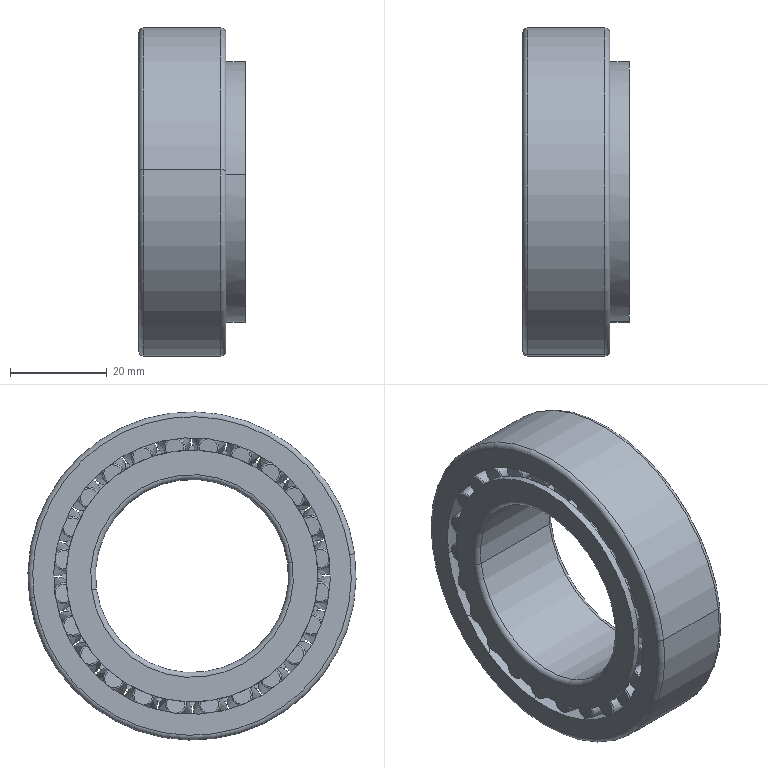Part | NX | features BREP 1 | 1 solid | 220 faces | box 22 x 68 x 68 mm | volume 39329 mm3 | torus 104 | cone 56 | plane 52 | cylinder 8 | commonest cylinder face diameters 40 x2 52.142 x2 54 x2 68 x2